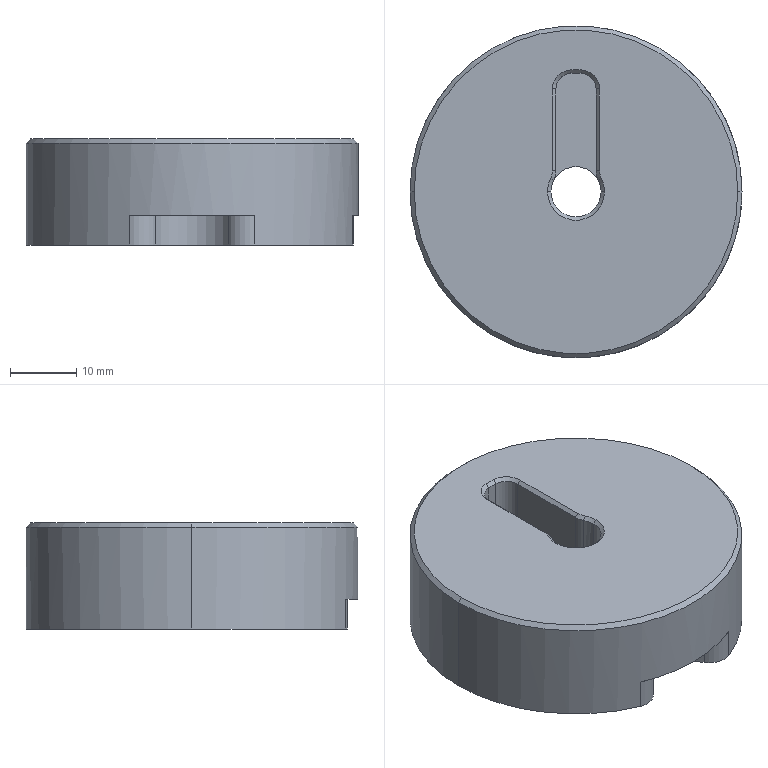NC program | NX | posted with a generic post | part box 50.292 x 50.292 x 16.057 mm
Whole program:
N10 G17 G21 G94 G90
(ZLEVEL_PROFILE_COPY_1 , TOOL : D4)
N12 T04 M6
N14 G54
N16 G17 G0 G90 X-0.549 Y-1.167 S4000 M3
N18 G43 Z30. H4
N20 Z-0.198
N22 G94 G1 X0.331 Y-1.893 F1000.
N24 G3 X0.726 Y-1.959 R0.4
N26 G1 X0.949 Y-1.862 F1500.
N28 G2 X3.172 Y-1.328 R4.895
N30 G1 X15.574
N32 G3 X16.234 Y-0.698 R0.661
N34 X16.234 Y0.698 R14.98
N36 X15.574 Y1.328 R0.661
N38 G1 X3.172
N40 G2 X0.93 Y1.872 R4.895
N42 G1 X0.76 Y1.946
N44 X0.734 Y1.956
N46 G3 X0.339 Y1.895 R0.4
N48 G1 X-0.584 Y1.15
N50 G0 X0.051 Y-1.09 Z-0.397
N52 G1 X0.08 Y-1.724 F1000.
N54 G3 X0.465 Y-1.833 R0.4
N56 X0.859 Y-1.685 R1.89 F1500.
N58 G2 X3.172 Y-1.129 R5.094
N60 G1 X15.574
N62 G3 X16.036 Y-0.688 R0.462
N64 X16.036 Y0.688 R14.782
N66 X15.574 Y1.129 R0.462
N68 G1 X3.172
N70 G2 X0.859 Y1.685 R5.094
N72 G1 X0.647 Y1.777
N74 G3 X0.25 Y1.732 R0.4
N76 G1 X0.156 Y1.08
N78 G0 X0.248 Y-0.948 Z-0.595
N80 G1 X0.409 Y-1.565 F1000.
N82 G3 X0.808 Y-1.586 R0.4
N84 G2 X3.172 Y-1.018 R5.205 F1500.
N86 G1 X15.574
N88 G3 X15.925 Y-0.683 R0.351
N90 X15.925 Y0.683 R14.67
N92 X15.574 Y1.018 R0.351
N94 G1 X3.172
N96 G2 X0.864 Y1.558 R5.205
N98 G1 X0.808 Y1.586
N100 G3 X0.409 Y1.563 R0.4
N102 G1 X0.248 Y0.948
N104 G0 Y-0.948 Z-0.794
N106 G1 X0.409 Y-1.565 F1000.
N108 G3 X0.808 Y-1.586 R0.4
N110 G2 X3.172 Y-1.018 R5.205 F1500.
N112 G1 X15.574
N114 G3 X15.925 Y-0.683 R0.351
N116 X15.925 Y0.683 R14.67
N118 X15.574 Y1.018 R0.351
N120 G1 X3.172
N122 G2 X0.864 Y1.558 R5.205
N124 G1 X0.808 Y1.586
N126 G3 X0.409 Y1.563 R0.4
N128 G1 X0.248 Y0.948
N130 G0 Y-0.948 Z-0.992
N132 G1 X0.409 Y-1.565 F1000.
N134 G3 X0.808 Y-1.586 R0.4
N136 G2 X3.172 Y-1.018 R5.205 F1500.
N138 G1 X15.574
N140 G3 X15.925 Y-0.683 R0.351
N142 X15.925 Y0.683 R14.67
N144 X15.574 Y1.018 R0.351
N146 G1 X3.172
N148 G2 X0.864 Y1.558 R5.205
N150 G1 X0.808 Y1.586
N152 G3 X0.409 Y1.563 R0.4
N154 G1 X0.248 Y0.948
N156 G0 Y-0.948 Z-1.191
N158 G1 X0.409 Y-1.565 F1000.
N160 G3 X0.808 Y-1.586 R0.4
N162 G2 X3.172 Y-1.018 R5.205 F1500.
N164 G1 X15.574
N166 G3 X15.925 Y-0.683 R0.351
N168 X15.925 Y0.683 R14.67
N170 X15.574 Y1.018 R0.351
N172 G1 X3.172
N174 G2 X0.864 Y1.558 R5.205
N176 G1 X0.808 Y1.586
N178 G3 X0.409 Y1.563 R0.4
N180 G1 X0.248 Y0.948
N182 G0 Y-0.948 Z-1.389
N184 G1 X0.409 Y-1.565 F1000.
N186 G3 X0.808 Y-1.586 R0.4
N188 G2 X3.172 Y-1.018 R5.205 F1500.
N190 G1 X15.574
N192 G3 X15.925 Y-0.683 R0.351
N194 X15.925 Y0.683 R14.67
N196 X15.574 Y1.018 R0.351
N198 G1 X3.172
N200 G2 X0.864 Y1.558 R5.205
N202 G1 X0.808 Y1.586
N204 G3 X0.409 Y1.563 R0.4
N206 G1 X0.248 Y0.948
N208 G0 Y-0.948 Z-1.588
N210 G1 X0.409 Y-1.565 F1000.
N212 G3 X0.808 Y-1.586 R0.4
N214 G2 X3.172 Y-1.018 R5.205 F1500.
N216 G1 X15.574
N218 G3 X15.925 Y-0.683 R0.351
N220 X15.925 Y0.683 R14.67
N222 X15.574 Y1.018 R0.351
N224 G1 X3.172
N226 G2 X0.864 Y1.558 R5.205
N228 G1 X0.808 Y1.586
N230 G3 X0.409 Y1.563 R0.4
N232 G1 X0.248 Y0.948
N234 G0 Y-0.948 Z-1.786
N236 G1 X0.409 Y-1.565 F1000.
N238 G3 X0.808 Y-1.586 R0.4
N240 G2 X3.172 Y-1.018 R5.205 F1500.
N242 G1 X15.574
N244 G3 X15.925 Y-0.683 R0.351
N246 X15.925 Y0.683 R14.67
N248 X15.574 Y1.018 R0.351
N250 G1 X3.172
N252 G2 X0.864 Y1.558 R5.205
N254 G1 X0.808 Y1.586
N256 G3 X0.409 Y1.563 R0.4
N258 G1 X0.248 Y0.948
N260 G0 Y-0.948 Z-1.984
N262 G1 X0.409 Y-1.565 F1000.
N264 G3 X0.808 Y-1.586 R0.4
N266 G2 X3.172 Y-1.018 R5.205 F1500.
N268 G1 X15.574
N270 G3 X15.925 Y-0.683 R0.351
N272 X15.925 Y0.683 R14.67
N274 X15.574 Y1.018 R0.351
N276 G1 X3.172
N278 G2 X0.864 Y1.558 R5.205
N280 G1 X0.808 Y1.586
N282 G3 X0.409 Y1.563 R0.4
N284 G1 X0.248 Y0.948
N286 G0 Y-0.948 Z-2.183
N288 G1 X0.409 Y-1.565 F1000.
N290 G3 X0.808 Y-1.586 R0.4
N292 G2 X3.172 Y-1.018 R5.205 F1500.
N294 G1 X15.574
N296 G3 X15.925 Y-0.683 R0.351
N298 X15.925 Y0.683 R14.67
N300 X15.574 Y1.018 R0.351
N302 G1 X3.172
N304 G2 X0.864 Y1.558 R5.205
N306 G1 X0.808 Y1.586
N308 G3 X0.409 Y1.563 R0.4
N310 G1 X0.248 Y0.948
N312 G0 Y-0.948 Z-2.381
N314 G1 X0.409 Y-1.565 F1000.
N316 G3 X0.808 Y-1.586 R0.4
N318 G2 X3.172 Y-1.018 R5.205 F1500.
N320 G1 X15.574
N322 G3 X15.925 Y-0.683 R0.351
N324 X15.925 Y0.683 R14.67
N326 X15.574 Y1.018 R0.351
N328 G1 X3.172
N330 G2 X0.864 Y1.558 R5.205
N332 G1 X0.808 Y1.586
N334 G3 X0.409 Y1.563 R0.4
N336 G1 X0.248 Y0.948
N338 G0 Y-0.948 Z-2.58
N340 G1 X0.409 Y-1.565 F1000.
N342 G3 X0.808 Y-1.586 R0.4
N344 G2 X3.172 Y-1.018 R5.205 F1500.
N346 G1 X15.574
N348 G3 X15.925 Y-0.683 R0.351
N350 X15.925 Y0.683 R14.67
N352 X15.574 Y1.018 R0.351
N354 G1 X3.172
N356 G2 X0.864 Y1.558 R5.205
N358 G1 X0.808 Y1.586
N360 G3 X0.409 Y1.563 R0.4
N362 G1 X0.248 Y0.948
N364 G0 Y-0.948 Z-2.778
N366 G1 X0.409 Y-1.565 F1000.
N368 G3 X0.808 Y-1.586 R0.4
N370 G2 X3.172 Y-1.018 R5.205 F1500.
N372 G1 X15.574
N374 G3 X15.925 Y-0.683 R0.351
N376 X15.925 Y0.683 R14.67
N378 X15.574 Y1.018 R0.351
N380 G1 X3.172
N382 G2 X0.864 Y1.558 R5.205
N384 G1 X0.808 Y1.586
N386 G3 X0.409 Y1.563 R0.4
N388 G1 X0.248 Y0.948
N390 G0 Y-0.948 Z-2.977
N392 G1 X0.409 Y-1.565 F1000.
N394 G3 X0.808 Y-1.586 R0.4
N396 G2 X3.172 Y-1.018 R5.205 F1500.
N398 G1 X15.574
N400 G3 X15.925 Y-0.683 R0.351
N402 X15.925 Y0.683 R14.67
N404 X15.574 Y1.018 R0.351
N406 G1 X3.172
N408 G2 X0.864 Y1.558 R5.205
N410 G1 X0.808 Y1.586
N412 G3 X0.409 Y1.563 R0.4
N414 G1 X0.248 Y0.948
N416 G0 Y-0.948 Z-3.175
N418 G1 X0.409 Y-1.565 F1000.
N420 G3 X0.808 Y-1.586 R0.4
N422 G2 X3.172 Y-1.018 R5.205 F1500.
N424 G1 X15.574
N426 G3 X15.925 Y-0.683 R0.351
N428 X15.925 Y0.683 R14.67
N430 X15.574 Y1.018 R0.351
N432 G1 X3.172
N434 G2 X0.864 Y1.558 R5.205
N436 G1 X0.808 Y1.586
N438 G3 X0.409 Y1.563 R0.4
N440 G1 X0.248 Y0.948
N442 G0 Y-0.948 Z-3.373
N444 G1 X0.409 Y-1.565 F1000.
N446 G3 X0.808 Y-1.586 R0.4
N448 G2 X3.172 Y-1.018 R5.205 F1500.
N450 G1 X15.574
N452 G3 X15.925 Y-0.683 R0.351
N454 X15.925 Y0.683 R14.67
N456 X15.574 Y1.018 R0.351
N458 G1 X3.172
N460 G2 X0.864 Y1.558 R5.205
N462 G1 X0.808 Y1.586
N464 G3 X0.409 Y1.563 R0.4
N466 G1 X0.248 Y0.948
N468 G0 Y-0.948 Z-3.572
N470 G1 X0.409 Y-1.565 F1000.
N472 G3 X0.808 Y-1.586 R0.4
N474 G2 X3.172 Y-1.018 R5.205 F1500.
N476 G1 X15.574
N478 G3 X15.925 Y-0.683 R0.351
N480 X15.925 Y0.683 R14.67
N482 X15.574 Y1.018 R0.351
N484 G1 X3.172
N486 G2 X0.864 Y1.558 R5.205
N488 G1 X0.808 Y1.586
N490 G3 X0.409 Y1.563 R0.4
N492 G1 X0.248 Y0.948
N494 G0 Y-0.948 Z-3.77
N496 G1 X0.409 Y-1.565 F1000.
N498 G3 X0.808 Y-1.586 R0.4
N500 G2 X3.172 Y-1.018 R5.205 F1500.
N502 G1 X15.574
N504 G3 X15.925 Y-0.683 R0.351
N506 X15.925 Y0.683 R14.67
N508 X15.574 Y1.018 R0.351
N510 G1 X3.172
N512 G2 X0.864 Y1.558 R5.205
N514 G1 X0.808 Y1.586
N516 G3 X0.409 Y1.563 R0.4
N518 G1 X0.248 Y0.948
N520 G0 Y-0.948 Z-3.969
N522 G1 X0.409 Y-1.565 F1000.
N524 G3 X0.808 Y-1.586 R0.4
N526 G2 X3.172 Y-1.018 R5.205 F1500.
N528 G1 X15.574
N530 G3 X15.925 Y-0.683 R0.351
N532 X15.925 Y0.683 R14.67
N534 X15.574 Y1.018 R0.351
N536 G1 X3.172
N538 G2 X0.864 Y1.558 R5.205
N540 G1 X0.808 Y1.586
N542 G3 X0.409 Y1.563 R0.4
N544 G1 X0.248 Y0.948
N546 G0 Y-0.948 Z-4.167
N548 G1 X0.409 Y-1.565 F1000.
N550 G3 X0.808 Y-1.586 R0.4
N552 G2 X3.172 Y-1.018 R5.205 F1500.
N554 G1 X15.574
N556 G3 X15.925 Y-0.683 R0.351
N558 X15.925 Y0.683 R14.67
N560 X15.574 Y1.018 R0.351
N562 G1 X3.172
N564 G2 X0.864 Y1.558 R5.205
N566 G1 X0.808 Y1.586
N568 G3 X0.409 Y1.563 R0.4
N570 G1 X0.248 Y0.948
N572 G0 Y-0.948 Z-4.366
N574 G1 X0.409 Y-1.565 F1000.
N576 G3 X0.808 Y-1.586 R0.4
N578 G2 X3.172 Y-1.018 R5.205 F1500.
N580 G1 X15.574
N582 G3 X15.925 Y-0.683 R0.351
N584 X15.925 Y0.683 R14.67
N586 X15.574 Y1.018 R0.351
N588 G1 X3.172
N590 G2 X0.864 Y1.558 R5.205
N592 G1 X0.808 Y1.586
N594 G3 X0.409 Y1.563 R0.4
N596 G1 X0.248 Y0.948
N598 G0 Y-0.948 Z-4.564
N600 G1 X0.409 Y-1.565 F1000.
N602 G3 X0.808 Y-1.586 R0.4
N604 G2 X3.172 Y-1.018 R5.205 F1500.
N606 G1 X15.574
N608 G3 X15.925 Y-0.683 R0.351
N610 X15.925 Y0.683 R14.67
N612 X15.574 Y1.018 R0.351
N614 G1 X3.172
N616 G2 X0.864 Y1.558 R5.205
N618 G1 X0.808 Y1.586
N620 G3 X0.409 Y1.563 R0.4
N622 G1 X0.248 Y0.948
N624 G0 Y-0.948 Z-4.763
N626 G1 X0.409 Y-1.565 F1000.
N628 G3 X0.808 Y-1.586 R0.4
N630 G2 X3.172 Y-1.018 R5.205 F1500.
N632 G1 X15.574
N634 G3 X15.925 Y-0.683 R0.351
N636 X15.925 Y0.683 R14.67
N638 X15.574 Y1.018 R0.351
N640 G1 X3.172
N642 G2 X0.864 Y1.558 R5.205
N644 G1 X0.808 Y1.586
N646 G3 X0.409 Y1.563 R0.4
N648 G1 X0.248 Y0.948
N650 G0 Y-0.948 Z-4.961
N652 G1 X0.409 Y-1.565 F1000.
N654 G3 X0.808 Y-1.586 R0.4
N656 G2 X3.172 Y-1.018 R5.205 F1500.
N658 G1 X15.574
N660 G3 X15.925 Y-0.683 R0.351
N662 X15.925 Y0.683 R14.67
N664 X15.574 Y1.018 R0.351
N666 G1 X3.172
N668 G2 X0.864 Y1.558 R5.205
N670 G1 X0.808 Y1.586
N672 G3 X0.409 Y1.563 R0.4
N674 G1 X0.248 Y0.948
N676 G0 Y-0.948 Z-5.159
N678 G1 X0.409 Y-1.565 F1000.
N680 G3 X0.808 Y-1.586 R0.4
N682 G2 X3.172 Y-1.018 R5.205 F1500.
N684 G1 X15.574
N686 G3 X15.925 Y-0.683 R0.351
N688 X15.925 Y0.683 R14.67
N690 X15.574 Y1.018 R0.351
N692 G1 X3.172
N694 G2 X0.864 Y1.558 R5.205
N696 G1 X0.808 Y1.586
N698 G3 X0.409 Y1.563 R0.4
N700 G1 X0.248 Y0.948
N702 G0 Y-0.948 Z-5.358
N704 G1 X0.409 Y-1.565 F1000.
N706 G3 X0.808 Y-1.586 R0.4
N708 G2 X3.172 Y-1.018 R5.205 F1500.
N710 G1 X15.574
N712 G3 X15.925 Y-0.683 R0.351
N714 X15.925 Y0.683 R14.67
N716 X15.574 Y1.018 R0.351
N718 G1 X3.172
N720 G2 X0.864 Y1.558 R5.205
N722 G1 X0.808 Y1.586
N724 G3 X0.409 Y1.563 R0.4
N726 G1 X0.248 Y0.948
N728 G0 Y-0.948 Z-5.556
N730 G1 X0.409 Y-1.565 F1000.
N732 G3 X0.808 Y-1.586 R0.4
N734 G2 X3.172 Y-1.018 R5.205 F1500.
N736 G1 X15.574
N738 G3 X15.925 Y-0.683 R0.351
N740 X15.925 Y0.683 R14.67
N742 X15.574 Y1.018 R0.351
N744 G1 X3.172
N746 G2 X0.864 Y1.558 R5.205
N748 G1 X0.808 Y1.586
N750 G3 X0.409 Y1.563 R0.4
N752 G1 X0.248 Y0.948
N754 G0 Y-0.948 Z-5.755
N756 G1 X0.409 Y-1.565 F1000.
N758 G3 X0.808 Y-1.586 R0.4
N760 G2 X3.172 Y-1.018 R5.205 F1500.
N762 G1 X15.574
N764 G3 X15.925 Y-0.683 R0.351
N766 X15.925 Y0.683 R14.67
N768 X15.574 Y1.018 R0.351
N770 G1 X3.172
N772 G2 X0.864 Y1.558 R5.205
N774 G1 X0.808 Y1.586
N776 G3 X0.409 Y1.563 R0.4
N778 G1 X0.248 Y0.948
N780 G0 Y-0.948 Z-5.953
N782 G1 X0.409 Y-1.565 F1000.
N784 G3 X0.808 Y-1.586 R0.4
N786 G2 X3.172 Y-1.018 R5.205 F1500.
N788 G1 X15.574
N790 G3 X15.925 Y-0.683 R0.351
N792 X15.925 Y0.683 R14.67
N794 X15.574 Y1.018 R0.351
N796 G1 X3.172
N798 G2 X0.864 Y1.558 R5.205
N800 G1 X0.808 Y1.586
N802 G3 X0.409 Y1.563 R0.4
N804 G1 X0.248 Y0.948
N806 G0 Y-0.948 Z-6.152
N808 G1 X0.409 Y-1.565 F1000.
N810 G3 X0.808 Y-1.586 R0.4
N812 G2 X3.172 Y-1.018 R5.205 F1500.
N814 G1 X15.574
N816 G3 X15.925 Y-0.683 R0.351
N818 X15.925 Y0.683 R14.67
N820 X15.574 Y1.018 R0.351
N822 G1 X3.172
N824 G2 X0.864 Y1.558 R5.205
N826 G1 X0.808 Y1.586
N828 G3 X0.409 Y1.563 R0.4
N830 G1 X0.248 Y0.948
N832 G0 Y-0.948 Z-6.35
N834 G1 X0.409 Y-1.565 F1000.
N836 G3 X0.808 Y-1.586 R0.4
N838 G2 X3.172 Y-1.018 R5.205 F1500.
N840 G1 X15.574
N842 G3 X15.925 Y-0.683 R0.351
N844 X15.925 Y0.683 R14.67
N846 X15.574 Y1.018 R0.351
N848 G1 X3.172
N850 G2 X0.864 Y1.558 R5.205
N852 G1 X0.808 Y1.586
N854 G3 X0.409 Y1.563 R0.4
N856 G1 X0.248 Y0.948
N858 G0 Y-0.948 Z-6.548
N860 G1 X0.409 Y-1.565 F1000.
N862 G3 X0.808 Y-1.586 R0.4
N864 G2 X3.172 Y-1.018 R5.205 F1500.
N866 G1 X15.574
N868 G3 X15.925 Y-0.683 R0.351
N870 X15.925 Y0.683 R14.67
N872 X15.574 Y1.018 R0.351
N874 G1 X3.172
N876 G2 X0.864 Y1.558 R5.205
N878 G1 X0.808 Y1.586
N880 G3 X0.409 Y1.563 R0.4
N882 G1 X0.248 Y0.948
N884 G0 Y-0.948 Z-6.747
N886 G1 X0.409 Y-1.565 F1000.
N888 G3 X0.808 Y-1.586 R0.4
N890 G2 X3.172 Y-1.018 R5.205 F1500.
N892 G1 X15.574
N894 G3 X15.925 Y-0.683 R0.351
N896 X15.925 Y0.683 R14.67
N898 X15.574 Y1.018 R0.351
N900 G1 X3.172
N902 G2 X0.864 Y1.558 R5.205
N904 G1 X0.808 Y1.586
N906 G3 X0.409 Y1.563 R0.4
N908 G1 X0.248 Y0.948
N910 G0 Y-0.948 Z-6.945
N912 G1 X0.409 Y-1.565 F1000.
N914 G3 X0.808 Y-1.586 R0.4
N916 G2 X3.172 Y-1.018 R5.205 F1500.
N918 G1 X15.574
N920 G3 X15.925 Y-0.683 R0.351
N922 X15.925 Y0.683 R14.67
N924 X15.574 Y1.018 R0.351
N926 G1 X3.172
N928 G2 X0.864 Y1.558 R5.205
N930 G1 X0.808 Y1.586
N932 G3 X0.409 Y1.563 R0.4
N934 G1 X0.248 Y0.948
N936 G0 Y-0.948 Z-7.144
N938 G1 X0.409 Y-1.565 F1000.
N940 G3 X0.808 Y-1.586 R0.4
N942 G2 X3.172 Y-1.018 R5.205 F1500.
N944 G1 X15.574
N946 G3 X15.925 Y-0.683 R0.351
N948 X15.925 Y0.683 R14.67
N950 X15.574 Y1.018 R0.351
N952 G1 X3.172
N954 G2 X0.864 Y1.558 R5.205
N956 G1 X0.808 Y1.586
N958 G3 X0.409 Y1.563 R0.4
N960 G1 X0.248 Y0.948
N962 G0 Y-0.948 Z-7.342
N964 G1 X0.409 Y-1.565 F1000.
N966 G3 X0.808 Y-1.586 R0.4
N968 G2 X3.172 Y-1.018 R5.205 F1500.
N970 G1 X15.574
N972 G3 X15.925 Y-0.683 R0.351
N974 X15.925 Y0.683 R14.67
N976 X15.574 Y1.018 R0.351
N978 G1 X3.172
N980 G2 X0.864 Y1.558 R5.205
N982 G1 X0.808 Y1.586
N984 G3 X0.409 Y1.563 R0.4
N986 G1 X0.248 Y0.948
N988 G0 Y-0.948 Z-7.541
N990 G1 X0.409 Y-1.565 F1000.
N992 G3 X0.808 Y-1.586 R0.4
N994 G2 X3.172 Y-1.018 R5.205 F1500.
N996 G1 X15.574
N998 G3 X15.925 Y-0.683 R0.351
N1000 X15.925 Y0.683 R14.67
N1002 X15.574 Y1.018 R0.351
N1004 G1 X3.172
N1006 G2 X0.864 Y1.558 R5.205
N1008 G1 X0.808 Y1.586
N1010 G3 X0.409 Y1.563 R0.4
N1012 G1 X0.248 Y0.948
N1014 G0 Y-0.948 Z-7.739
N1016 G1 X0.409 Y-1.565 F1000.
N1018 G3 X0.808 Y-1.586 R0.4
N1020 G2 X3.172 Y-1.018 R5.205 F1500.
N1022 G1 X15.574
N1024 G3 X15.925 Y-0.683 R0.351
N1026 X15.925 Y0.683 R14.67
N1028 X15.574 Y1.018 R0.351
N1030 G1 X3.172
N1032 G2 X0.864 Y1.558 R5.205
N1034 G1 X0.808 Y1.586
N1036 G3 X0.409 Y1.563 R0.4
N1038 G1 X0.248 Y0.948
N1040 G0 Y-0.948 Z-7.938
N1042 G1 X0.409 Y-1.565 F1000.
N1044 G3 X0.808 Y-1.586 R0.4
N1046 G2 X3.172 Y-1.018 R5.205 F1500.
N1048 G1 X15.574
N1050 G3 X15.925 Y-0.683 R0.351
N1052 X15.925 Y0.683 R14.67
N1054 X15.574 Y1.018 R0.351
N1056 G1 X3.172
N1058 G2 X0.864 Y1.558 R5.205
N1060 G1 X0.808 Y1.586
N1062 G3 X0.409 Y1.563 R0.4
N1064 G1 X0.248 Y0.948
N1066 G0 Y-0.948 Z-8.136
N1068 G1 X0.409 Y-1.565 F1000.
N1070 G3 X0.808 Y-1.586 R0.4
N1072 G2 X3.172 Y-1.018 R5.205 F1500.
N1074 G1 X15.574
N1076 G3 X15.925 Y-0.683 R0.351
N1078 X15.925 Y0.683 R14.67
N1080 X15.574 Y1.018 R0.351
N1082 G1 X3.172
N1084 G2 X0.864 Y1.558 R5.205
N1086 G1 X0.808 Y1.586
N1088 G3 X0.409 Y1.563 R0.4
N1090 G1 X0.248 Y0.948
N1092 G0 Y-0.948 Z-8.334
N1094 G1 X0.409 Y-1.565 F1000.
N1096 G3 X0.808 Y-1.586 R0.4
N1098 G2 X3.172 Y-1.018 R5.205 F1500.
N1100 G1 X15.574
N1102 G3 X15.925 Y-0.683 R0.351
N1104 X15.925 Y0.683 R14.67
N1106 X15.574 Y1.018 R0.351
N1108 G1 X3.172
N1110 G2 X0.864 Y1.558 R5.205
N1112 G1 X0.808 Y1.586
N1114 G3 X0.409 Y1.563 R0.4
N1116 G1 X0.248 Y0.948
N1118 G0 Y-0.948 Z-8.533
N1120 G1 X0.409 Y-1.565 F1000.
N1122 G3 X0.808 Y-1.586 R0.4
N1124 G2 X3.172 Y-1.018 R5.205 F1500.
N1126 G1 X15.574
N1128 G3 X15.925 Y-0.683 R0.351
N1130 X15.925 Y0.683 R14.67
N1132 X15.574 Y1.018 R0.351
N1134 G1 X3.172
N1136 G2 X0.864 Y1.558 R5.205
N1138 G1 X0.808 Y1.586
N1140 G3 X0.409 Y1.563 R0.4
N1142 G1 X0.248 Y0.948
N1144 G0 Y-0.948 Z-8.731
N1146 G1 X0.409 Y-1.565 F1000.
N1148 G3 X0.808 Y-1.586 R0.4
N1150 G2 X3.172 Y-1.018 R5.205 F1500.
N1152 G1 X15.574
N1154 G3 X15.925 Y-0.683 R0.351
N1156 X15.925 Y0.683 R14.67
N1158 X15.574 Y1.018 R0.351
N1160 G1 X3.172
N1162 G2 X0.864 Y1.558 R5.205
N1164 G1 X0.808 Y1.586
N1166 G3 X0.409 Y1.563 R0.4
N1168 G1 X0.248 Y0.948
N1170 G0 Y-0.948 Z-8.93
N1172 G1 X0.409 Y-1.565 F1000.
N1174 G3 X0.808 Y-1.586 R0.4
N1176 G2 X3.172 Y-1.018 R5.205 F1500.
N1178 G1 X15.574
N1180 G3 X15.925 Y-0.683 R0.351
N1182 X15.925 Y0.683 R14.67
N1184 X15.574 Y1.018 R0.351
N1186 G1 X3.172
N1188 G2 X0.864 Y1.558 R5.205
N1190 G1 X0.808 Y1.586
N1192 G3 X0.409 Y1.563 R0.4
N1194 G1 X0.248 Y0.948
N1196 G0 Y-0.948 Z-9.128
N1198 G1 X0.409 Y-1.565 F1000.
N1200 G3 X0.808 Y-1.586 R0.4
N1202 G2 X3.172 Y-1.018 R5.205 F1500.
N1204 G1 X15.574
N1206 G3 X15.925 Y-0.683 R0.351
N1208 X15.925 Y0.683 R14.67
N1210 X15.574 Y1.018 R0.351
N1212 G1 X3.172
N1214 G2 X0.864 Y1.558 R5.205
N1216 G1 X0.808 Y1.586
N1218 G3 X0.409 Y1.563 R0.4
N1220 G1 X0.248 Y0.948
N1222 G0 Y-0.948 Z-9.327
N1224 G1 X0.409 Y-1.565 F1000.
N1226 G3 X0.808 Y-1.586 R0.4
N1228 G2 X3.172 Y-1.018 R5.205 F1500.
N1230 G1 X15.574
N1232 G3 X15.925 Y-0.683 R0.351
N1234 X15.925 Y0.683 R14.67
N1236 X15.574 Y1.018 R0.351
N1238 G1 X3.172
N1240 G2 X0.864 Y1.558 R5.205
N1242 G1 X0.808 Y1.586
N1244 G3 X0.409 Y1.563 R0.4
N1246 G1 X0.248 Y0.948
N1248 G0 Y-0.948 Z-9.525
N1250 G1 X0.409 Y-1.565 F1000.
N1252 G3 X0.808 Y-1.586 R0.4
N1254 G2 X3.172 Y-1.018 R5.205 F1500.
N1256 G1 X15.574
N1258 G3 X15.925 Y-0.683 R0.351
N1260 X15.925 Y0.683 R14.67
N1262 X15.574 Y1.018 R0.351
N1264 G1 X3.172
N1266 G2 X0.864 Y1.558 R5.205
N1268 G1 X0.808 Y1.586
N1270 G3 X0.409 Y1.563 R0.4
N1272 G1 X0.248 Y0.948
N1274 G0 Y-0.948 Z-9.723
N1276 G1 X0.409 Y-1.565 F1000.
N1278 G3 X0.808 Y-1.586 R0.4
N1280 G2 X3.172 Y-1.018 R5.205 F1500.
N1282 G1 X15.574
N1284 G3 X15.925 Y-0.683 R0.351
N1286 X15.925 Y0.683 R14.67
N1288 X15.574 Y1.018 R0.351
N1290 G1 X3.172
N1292 G2 X0.864 Y1.558 R5.205
N1294 G1 X0.808 Y1.586
N1296 G3 X0.409 Y1.563 R0.4
N1298 G1 X0.248 Y0.948
N1300 G0 Y-0.948 Z-9.922
N1302 G1 X0.409 Y-1.565 F1000.
N1304 G3 X0.808 Y-1.586 R0.4
N1306 G2 X3.172 Y-1.018 R5.205 F1500.
N1308 G1 X15.574
N1310 G3 X15.925 Y-0.683 R0.351
N1312 X15.925 Y0.683 R14.67
N1314 X15.574 Y1.018 R0.351
N1316 G1 X3.172
N1318 G2 X0.864 Y1.558 R5.205
N1320 G1 X0.808 Y1.586
N1322 G3 X0.409 Y1.563 R0.4
N1324 G1 X0.248 Y0.948
N1326 G0 Y-0.948 Z-10.12
N1328 G1 X0.409 Y-1.565 F1000.
N1330 G3 X0.808 Y-1.586 R0.4
N1332 G2 X3.172 Y-1.018 R5.205 F1500.
N1334 G1 X15.574
N1336 G3 X15.925 Y-0.683 R0.351
N1338 X15.925 Y0.683 R14.67
N1340 X15.574 Y1.018 R0.351
N1342 G1 X3.172
N1344 G2 X0.864 Y1.558 R5.205
N1346 G1 X0.808 Y1.586
N1348 G3 X0.409 Y1.563 R0.4
N1350 G1 X0.248 Y0.948
N1352 G0 Y-0.948 Z-10.319
N1354 G1 X0.409 Y-1.565 F1000.
N1356 G3 X0.808 Y-1.586 R0.4
N1358 G2 X3.172 Y-1.018 R5.205 F1500.
N1360 G1 X15.574
N1362 G3 X15.925 Y-0.683 R0.351
N1364 X15.925 Y0.683 R14.67
N1366 X15.574 Y1.018 R0.351
N1368 G1 X3.172
N1370 G2 X0.864 Y1.558 R5.205
N1372 G1 X0.808 Y1.586
N1374 G3 X0.409 Y1.563 R0.4
N1376 G1 X0.248 Y0.948
N1378 G0 Y-0.948 Z-10.517
N1380 G1 X0.409 Y-1.565 F1000.
N1382 G3 X0.808 Y-1.586 R0.4
N1384 G2 X3.172 Y-1.018 R5.205 F1500.
N1386 G1 X15.574
N1388 G3 X15.925 Y-0.683 R0.351
N1390 X15.925 Y0.683 R14.67
N1392 X15.574 Y1.018 R0.351
N1394 G1 X3.172
N1396 G2 X0.864 Y1.558 R5.205
N1398 G1 X0.808 Y1.586
N1400 G3 X0.409 Y1.563 R0.4
N1402 G1 X0.248 Y0.948
N1404 G0 Y-0.948 Z-10.716
N1406 G1 X0.409 Y-1.565 F1000.
N1408 G3 X0.808 Y-1.586 R0.4
N1410 G2 X3.172 Y-1.018 R5.205 F1500.
N1412 G1 X15.574
N1414 G3 X15.925 Y-0.683 R0.351
N1416 X15.925 Y0.683 R14.67
N1418 X15.574 Y1.018 R0.351
N1420 G1 X3.172
N1422 G2 X0.864 Y1.558 R5.205
N1424 G1 X0.808 Y1.586
N1426 G3 X0.409 Y1.563 R0.4
N1428 G1 X0.248 Y0.948
N1430 G0 Y-0.948 Z-10.914
N1432 G1 X0.409 Y-1.565 F1000.
N1434 G3 X0.808 Y-1.586 R0.4
N1436 G2 X3.172 Y-1.018 R5.205 F1500.
N1438 G1 X15.574
N1440 G3 X15.925 Y-0.683 R0.351
N1442 X15.925 Y0.683 R14.67
N1444 X15.574 Y1.018 R0.351
N1446 G1 X3.172
N1448 G2 X0.864 Y1.558 R5.205
N1450 G1 X0.808 Y1.586
N1452 G3 X0.409 Y1.563 R0.4
N1454 G1 X0.248 Y0.948
N1456 G0 Y-0.948 Z-11.113
N1458 G1 X0.409 Y-1.565 F1000.
N1460 G3 X0.808 Y-1.586 R0.4
N1462 G2 X3.172 Y-1.018 R5.205 F1500.
N1464 G1 X15.574
N1466 G3 X15.925 Y-0.683 R0.351
N1468 X15.925 Y0.683 R14.67
N1470 X15.574 Y1.018 R0.351
N1472 G1 X3.172
N1474 G2 X0.864 Y1.558 R5.205
N1476 G1 X0.808 Y1.586
N1478 G3 X0.409 Y1.563 R0.4
N1480 G1 X0.248 Y0.948
N1482 G0 Z30.
N1484 M5
(ZLEVEL_PROFILE_COPY_COPY_1_COPY_COPY_COPY_1 , TOOL : D4JING)
N1486 T05 M6
N1488 G54
N1490 G17 G0 G90 X-0.351 Y-1.366 S4000 M3
N1492 G43 Z30. H5
N1494 Z-11.113
N1496 G94 G1 X-0.132 Y-1.645 F850.
N1498 G3 X0.239 Y-1.794 R0.4
N1500 X0.804 Y-1.621 R1.91
N1502 G1 X0.896 Y-1.576
N1504 G2 X3.172 Y-1.048 R5.175
N1506 G1 X15.574
N1508 G3 X15.955 Y-0.685 R0.381
N1510 X15.955 Y0.685 R14.7
N1512 X15.574 Y1.048 R0.381
N1514 G1 X3.172
N1516 G2 X0.886 Y1.58 R5.175
N1518 G1 X0.805 Y1.621
N1520 G3 X0.24 Y1.794 R1.788
N1522 X-0.13 Y1.641 R0.4
N1524 G1 X-0.339 Y1.369
N1526 G0 Z30.
N1528 M5
(PLANAR_MILL , TOOL : D4_CHAMFER-MILL)
N1530 T03 M6
N1532 G54
N1534 G17 G0 G90 X9.973 Y1.306 S4000 M3
N1536 G43 Z30. H3
N1538 Z0.7
N1540 G94 G1 Z-0.8 F1000.
N1542 G3 X9.373 Y1.506 R1.
N1544 G1 X3.172
N1546 G2 X1.03 Y2.021 R4.717
N1548 G3 X1.03 Y-2.021 R-2.268
N1550 G2 X3.172 Y-1.506 R4.717
N1552 G1 X15.574
N1554 G3 X16.412 Y-0.706 R0.839
N1556 X16.412 Y0.706 R15.158
N1558 X15.574 Y1.506 R0.839
N1560 G1 X9.373
N1562 G3 X8.773 Y1.306 R1.
N1564 G1 X10.208
N1566 G3 X9.373 Y1.756 R1.
N1568 G1 X3.172
N1570 G2 X1.144 Y2.243 R4.467
N1572 G3 X1.144 Y-2.243 R-2.518
N1574 G2 X3.172 Y-1.756 R4.467
N1576 G1 X15.574
N1578 G3 X16.662 Y-0.717 R1.089
N1580 X16.662 Y0.717 R15.409
N1582 X15.574 Y1.756 R1.089
N1584 G1 X9.373
N1586 G3 X8.773 Y1.556 R1.
N1588 G1 Z0.7
N1590 G0 Z30.
N1592 M5
N1594 M2